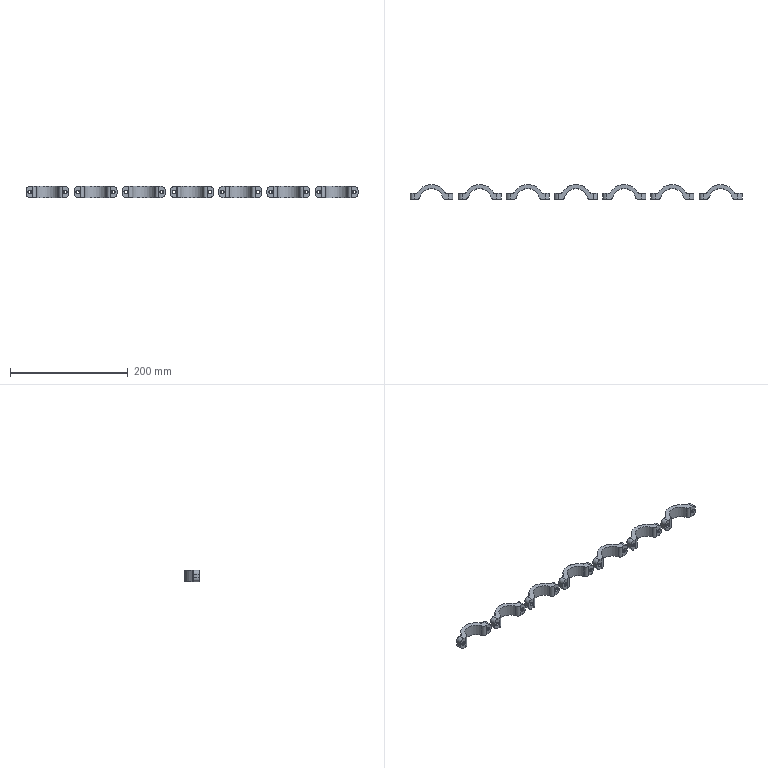Part | 8 solids | 288 faces | volume 104191 mm3 | cylinder 112 | plane 80 | cone 64 | other 32 | commonest cylinder face diameters 5 x32 6.8 x32 14 x32 40.1 x8 54.1 x8